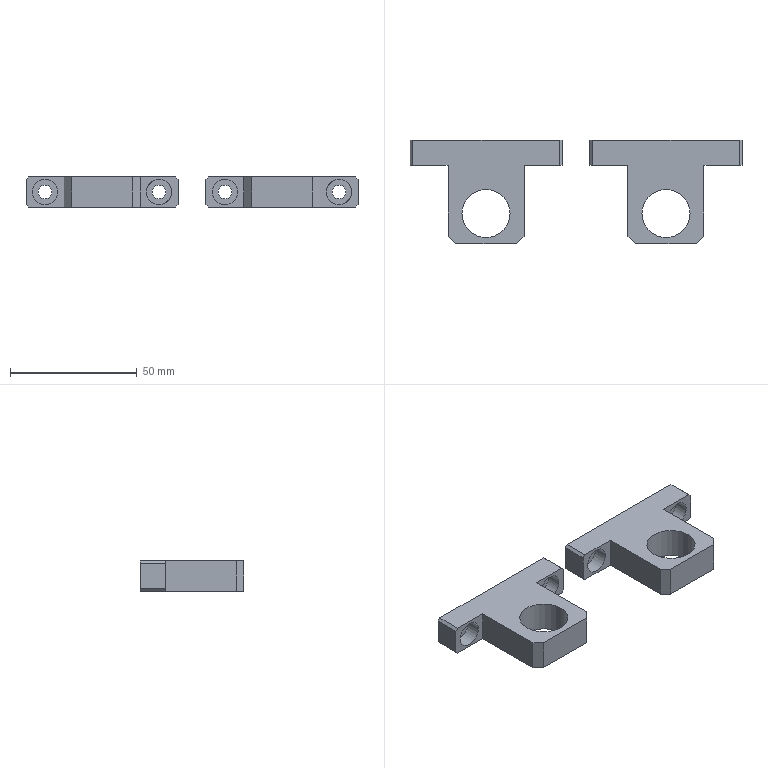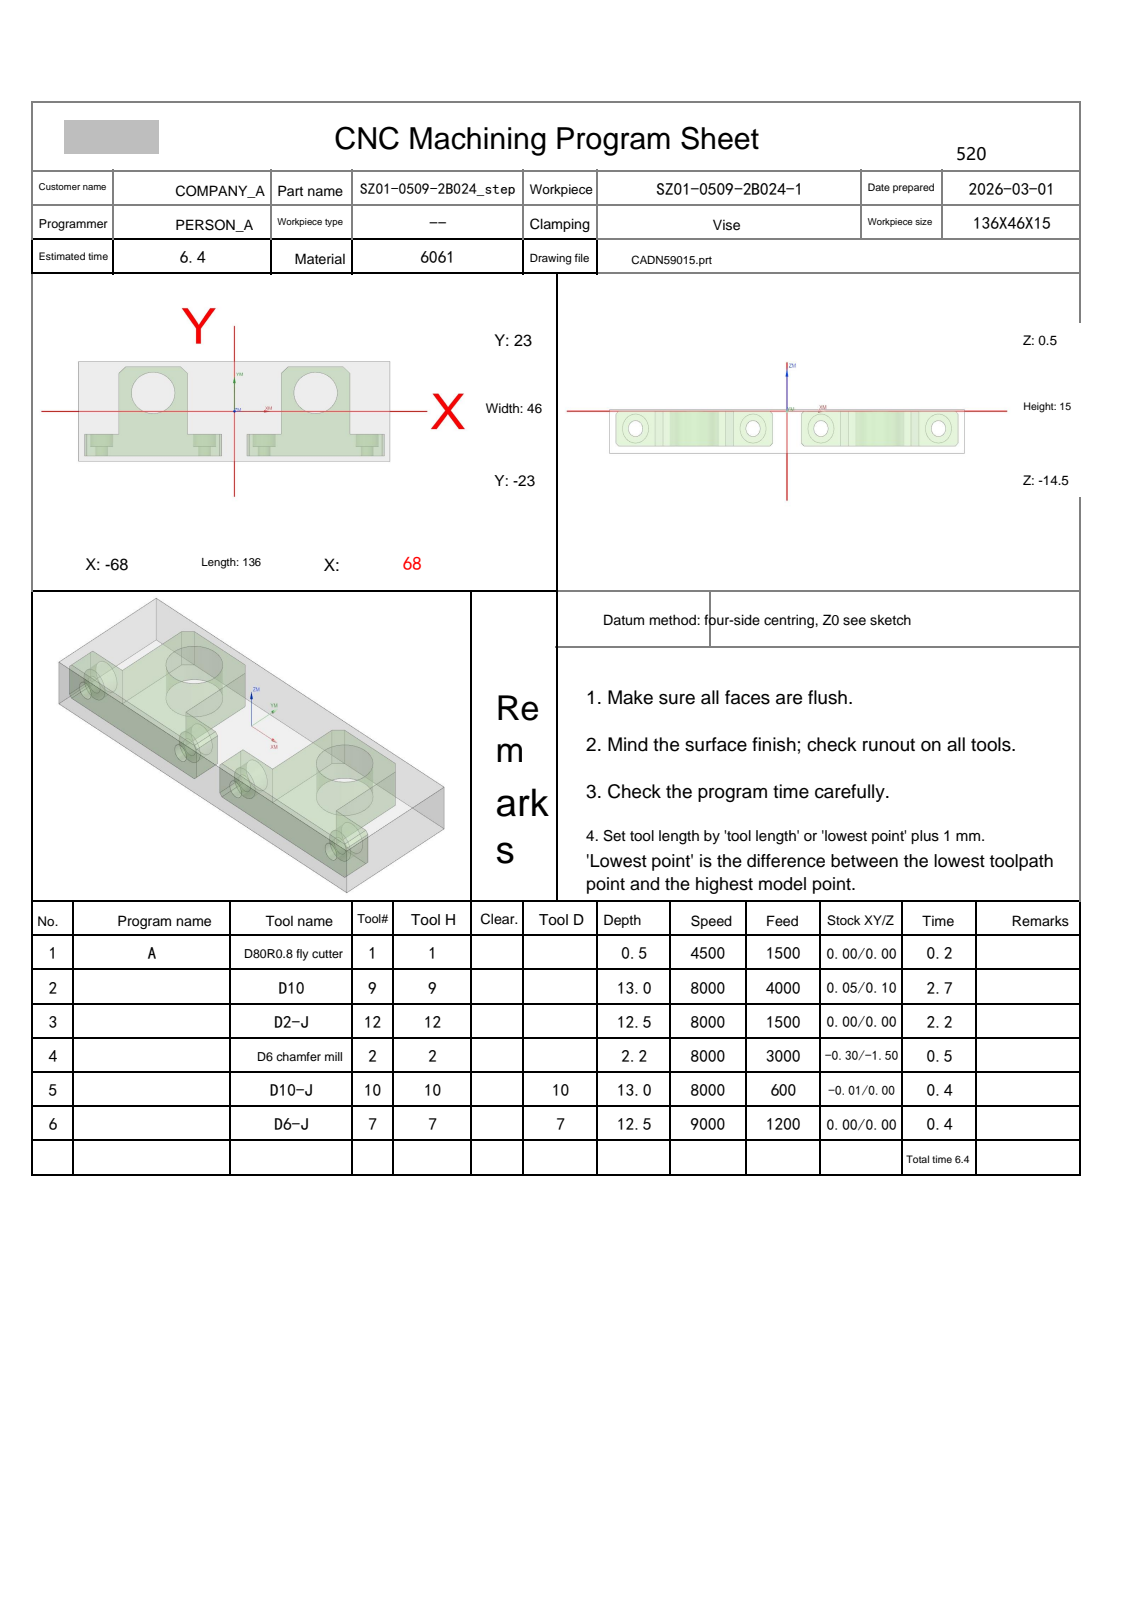NC program | NX | posted by the shop | part box 131 x 41 x 12 mm
Lines 8093 to 8452 of 8452:
N4 T02 M06
(D6 chamfer mill  D=6. R=0. H=02 ce=0.00 di=0.00)
G00 G90 G54 X35.5 Y8.5 M03 S8000
G43 H02 Z50.
M08
G98 G81 X35.5 Y8.5 Z-.8 R1. F500.
X-35.5
G80
G00 Z50.
G00 G90 X6.039 Y-9.293 M03 S8000
Z50.
Z2.935
G01 Z-1.5 F3000.
X6.211 Y-9.233
X6.5 Y-9.2
X19.2
Y17.5
X19.225 Y17.754
X19.299 Y17.997
X19.419 Y18.222
X19.581 Y18.419
X22.581 Y21.419
X22.778 Y21.581
X23.003 Y21.701
X23.246 Y21.775
X23.5 Y21.8
X47.5
X47.754 Y21.775
X47.997 Y21.701
X48.222 Y21.581
X48.419 Y21.419
X51.419 Y18.419
X51.581 Y18.222
X51.701 Y17.997
X51.775 Y17.754
X51.8 Y17.5
Y-9.2
X64.5
X64.789 Y-9.233
X64.961 Y-9.293
Z2.935
G00 Z50.
Y-21.707
Z2.935
G01 Z-1.5
X64.789 Y-21.767
X64.5 Y-21.8
X35.5
X6.5
X6.211 Y-21.767
X6.039 Y-21.707
Z2.935
G00 Z50.
X28.115 Y8.789
Z2.122
G01 Z-1.5
G03 X27.84 Y8.855 I-.275 J-.533
X27.307 Y8.53 I0.0 J-.6
G01 X27.3 Y8.5
G03 X35.5 Y.3 I8.2 J0.0
X43.7 Y8.5 I0.0 J8.2
X35.5 Y16.7 I-8.2 J0.0
X27.3 Y8.5 I0.0 J-8.2
G01 X27.307 Y8.47
G03 X27.84 Y8.145 I.533 J.275
X28.115 Y8.211 I0.0 J.6
G01 Z2.122
G00 Z50.
X-64.961 Y-9.293
Z2.935
G01 Z-1.5
X-64.789 Y-9.233
X-64.5 Y-9.2
X-51.8
Y17.5
X-51.775 Y17.754
X-51.701 Y17.997
X-51.581 Y18.222
X-51.419 Y18.419
X-48.419 Y21.419
X-48.222 Y21.581
X-47.997 Y21.701
X-47.754 Y21.775
X-47.5 Y21.8
X-23.5
X-23.246 Y21.775
X-23.003 Y21.701
X-22.778 Y21.581
X-22.581 Y21.419
X-19.581 Y18.419
X-19.419 Y18.222
X-19.299 Y17.997
X-19.225 Y17.754
X-19.2 Y17.5
Y-9.2
X-6.5
X-6.211 Y-9.233
X-6.039 Y-9.293
Z2.935
G00 Z50.
Y-21.707
Z2.935
G01 Z-1.5
X-6.211 Y-21.767
X-6.5 Y-21.8
X-35.5
X-64.5
X-64.789 Y-21.767
X-64.961 Y-21.707
Z2.935
G00 Z50.
X-42.885 Y8.789
Z2.122
G01 Z-1.5
G03 X-43.16 Y8.855 I-.275 J-.533
X-43.693 Y8.53 I0.0 J-.6
G01 X-43.7 Y8.5
G03 X-35.5 Y.3 I8.2 J0.0
X-27.3 Y8.5 I0.0 J8.2
X-35.5 Y16.7 I-8.2 J0.0
X-43.7 Y8.5 I0.0 J-8.2
G01 X-43.693 Y8.47
G03 X-43.16 Y8.145 I.533 J.275
X-42.885 Y8.211 I0.0 J.6
G01 Z2.122
G00 Z50.
G00 G90 X30.2 Y11.5 M03 S8000
Z50.
Z-1.
G01 Z-1.5 F1000.
G03 X27.2 Y8.5 I0.0 J-3.
X35.5 Y.2 I8.3 J0.0
X43.8 Y8.5 I0.0 J8.3
X35.5 Y16.8 I-8.3 J0.0
X27.2 Y8.5 I0.0 J-8.3
X30.2 Y5.5 I3. J0.0
G01 Z-1.
G00 Z50.
X-40.8 Y11.5
Z-1.
G01 Z-1.5
G03 X-43.8 Y8.5 I0.0 J-3.
X-35.5 Y.2 I8.3 J0.0
X-27.2 Y8.5 I0.0 J8.3
X-35.5 Y16.8 I-8.3 J0.0
X-43.8 Y8.5 I0.0 J-8.3
X-40.8 Y5.5 I3. J0.0
G01 Z-1.
G00 Z50.
G00 G90 X-66.208 Y-23.4 M03 S6500
Z50.
Z-.2
G01 Z-1.7 F1500.
X-66.199 Y-23.332
X-66.2 Y-23.263
Y-7.737
X-66.199 Y-7.668
X-66.208 Y-7.6
Z-.2
G00 Z50.
X-4.792
Z-.2
G01 Z-1.7
X-4.801 Y-7.668
X-4.8 Y-7.737
Y-23.263
X-4.801 Y-23.332
X-4.792 Y-23.4
Z-.2
G00 X4.792
G01 Z-1.7
X4.801 Y-23.332
X4.8 Y-23.263
Y-7.737
X4.801 Y-7.668
X4.792 Y-7.6
Z-.2
G00 Z50.
X66.208
Z-.2
G01 Z-1.7
X66.199 Y-7.668
X66.2 Y-7.737
Y-23.263
X66.199 Y-23.332
X66.208 Y-23.4
Z-.2
G00 Z50.
G91 G28 Z0.0
M05
M09
G91 G28 Z0.0
M01
N5 T10 M06
(D10-J  D=10. R=0. H=10 ce=-0.01 di=0.00)
G00 G90 G54 X-31.719 Y6.099 M03 S8000
G43 H10 Z50.
M08
Z.5
G01 X-31.652 Y6.197 Z.494 F600.
X-31.398 Y6.686 Z.465
X-31.207 Y7.203 Z.436
X-31.08 Y7.74 Z.407
X-31.02 Y8.288 Z.378
Y8.712 Z.356
X-31.088 Y9.306 Z.325
X-31.235 Y9.886 Z.293
X-31.457 Y10.441 Z.262
X-31.752 Y10.962 Z.231
X-32.113 Y11.439 Z.199
X-32.534 Y11.864 Z.168
X-33.008 Y12.229 Z.137
X-33.527 Y12.527 Z.105
X-34.08 Y12.754 Z.074
X-34.659 Y12.905 Z.042
X-35.253 Y12.978 Z.011
X-35.465 Y12.98 Z0.0
G41 D10
X-35.5 Y13.015
G03 X-40.015 Y8.5 Z-1.042 I0.0 J-4.515
X-35.5 Y3.985 Z-2.083 I4.515 J0.0
X-30.985 Y8.5 Z-3.125 I0.0 J4.515
X-35.5 Y13.015 Z-4.167 I-4.515 J0.0
X-40.015 Y8.5 Z-5.208 I0.0 J-4.515
X-35.5 Y3.985 Z-6.25 I4.515 J0.0
X-30.985 Y8.5 Z-7.292 I0.0 J4.515
X-35.5 Y13.015 Z-8.333 I-4.515 J0.0
X-40.015 Y8.5 Z-9.375 I0.0 J-4.515
X-35.5 Y3.985 Z-10.417 I4.515 J0.0
X-30.985 Y8.5 Z-11.458 I0.0 J4.515
X-35.5 Y13.015 Z-12.5 I-4.515 J0.0
X-40.015 Y8.5 I0.0 J-4.515
X-35.5 Y3.985 I4.515 J0.0
X-30.985 Y8.5 I0.0 J4.515
X-35.5 Y13.015 I-4.515 J0.0
X-35.899 Y12.997 I0.0 J-4.515
G01 X-35.927 Y12.993
X-35.945 Y12.971
Y12.943
G40 X-35.94 Y12.893
Z-11.5
G00 Z50.
X39.281 Y6.099
Z.5
G01 X39.348 Y6.197 Z.494
X39.602 Y6.686 Z.465
X39.793 Y7.203 Z.436
X39.92 Y7.74 Z.407
X39.98 Y8.288 Z.378
Y8.712 Z.356
X39.912 Y9.306 Z.325
X39.765 Y9.886 Z.293
X39.543 Y10.441 Z.262
X39.248 Y10.962 Z.231
X38.887 Y11.439 Z.199
X38.466 Y11.864 Z.168
X37.992 Y12.229 Z.137
X37.473 Y12.527 Z.105
X36.92 Y12.754 Z.074
X36.341 Y12.905 Z.042
X35.747 Y12.978 Z.011
X35.535 Y12.98 Z0.0
G41 D10
X35.5 Y13.015
G03 X30.985 Y8.5 Z-1.042 I0.0 J-4.515
X35.5 Y3.985 Z-2.083 I4.515 J0.0
X40.015 Y8.5 Z-3.125 I0.0 J4.515
X35.5 Y13.015 Z-4.167 I-4.515 J0.0
X30.985 Y8.5 Z-5.208 I0.0 J-4.515
X35.5 Y3.985 Z-6.25 I4.515 J0.0
X40.015 Y8.5 Z-7.292 I0.0 J4.515
X35.5 Y13.015 Z-8.333 I-4.515 J0.0
X30.985 Y8.5 Z-9.375 I0.0 J-4.515
X35.5 Y3.985 Z-10.417 I4.515 J0.0
X40.015 Y8.5 Z-11.458 I0.0 J4.515
X35.5 Y13.015 Z-12.5 I-4.515 J0.0
X30.985 Y8.5 I0.0 J-4.515
X35.5 Y3.985 I4.515 J0.0
X40.015 Y8.5 I0.0 J4.515
X35.5 Y13.015 I-4.515 J0.0
X35.101 Y12.997 I0.0 J-4.515
G01 X35.073 Y12.993
X35.055 Y12.971
Y12.943
G40 X35.06 Y12.893
Z-11.5
G00 Z50.
G91 G28 Z0.0
M05
M09
G91 G28 Z0.0
M01
N6 T07 M06
(D6-J  D=6. R=0. H=07 ce=0.00 di=0.00)
G00 G90 G54 X66.517 Y-24.573 M03 S9000
G43 H07 Z50.
M08
Z-11.5
G01 Z-12. F1200.
G41 D07
X66.492 Y-24.375
G03 X65.5 Y-23.5 I-.992 J-.125
G01 X5.5
G02 X2.5 Y-20.5 I0.0 J3.
G01 Y-10.5
G02 X5.5 Y-7.5 I3. J0.0
G01 X17.5
Y17.5
G02 X18.379 Y19.621 I3. J0.0
G01 X21.379 Y22.621
G02 X23.5 Y23.5 I2.121 J-2.121
G01 X47.5
G02 X49.621 Y22.621 I0.0 J-3.
G01 X52.621 Y19.621
G02 X53.5 Y17.5 I-2.121 J-2.121
G01 Y-7.5
X65.5
G02 X68.5 Y-10.5 I0.0 J-3.
G01 Y-20.5
G02 X65.5 Y-23.5 I-3. J0.0
G01 X65.
G03 X64. Y-24.5 I0.0 J-1.
G01 G40 Y-24.7
Z-11.5
G00 Z50.
X-4.483 Y-24.573
Z-11.5
G01 Z-12.
G41 D07
X-4.508 Y-24.375
G03 X-5.5 Y-23.5 I-.992 J-.125
G01 X-65.5
G02 X-68.5 Y-20.5 I0.0 J3.
G01 Y-10.5
G02 X-65.5 Y-7.5 I3. J0.0
G01 X-53.5
Y17.5
G02 X-52.621 Y19.621 I3. J0.0
G01 X-49.621 Y22.621
G02 X-47.5 Y23.5 I2.121 J-2.121
G01 X-23.5
G02 X-21.379 Y22.621 I0.0 J-3.
G01 X-18.379 Y19.621
G02 X-17.5 Y17.5 I-2.121 J-2.121
G01 Y-7.5
X-5.5
G02 X-2.5 Y-10.5 I0.0 J-3.
G01 Y-20.5
G02 X-5.5 Y-23.5 I-3. J0.0
G01 X-6.
G03 X-7. Y-24.5 I0.0 J-1.
G01 G40 Y-24.7
Z-11.5
G00 Z50.
M05
M09
G91 G28 Z0.0
G91 G28 Y0.0
M30
%